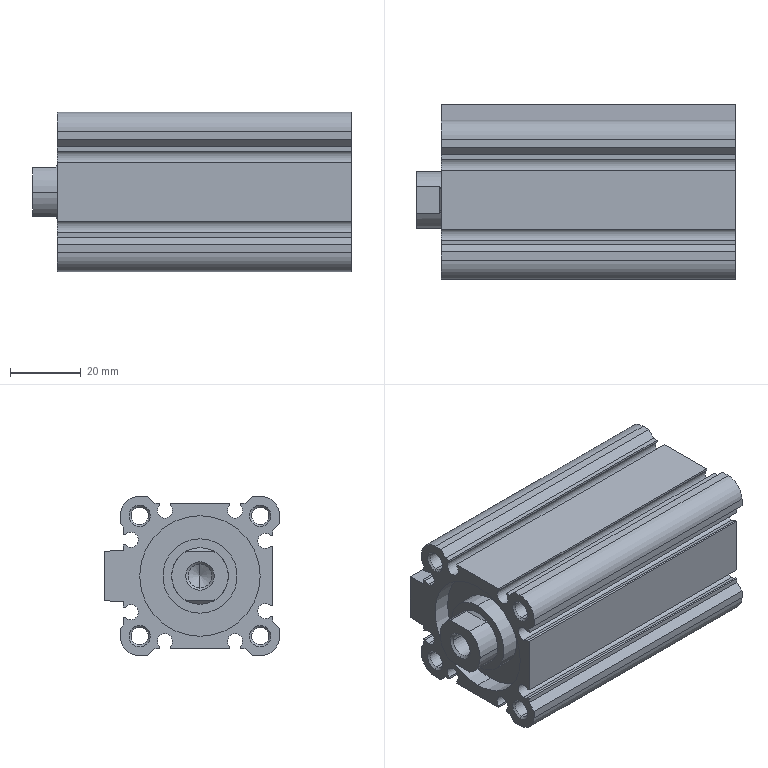Part | STEP file | Slim cylinder CDQ2A32-50DZ_with magnet | 2 solids | 162 faces | box 90 x 49.5 x 45 mm | volume 103379 mm3 | plane 72 | cylinder 66 | cone 24 | commonest cylinder face diameters 4.26 x18 4.917 x16 6 x8 8.566 x4 11 x4 16 x4